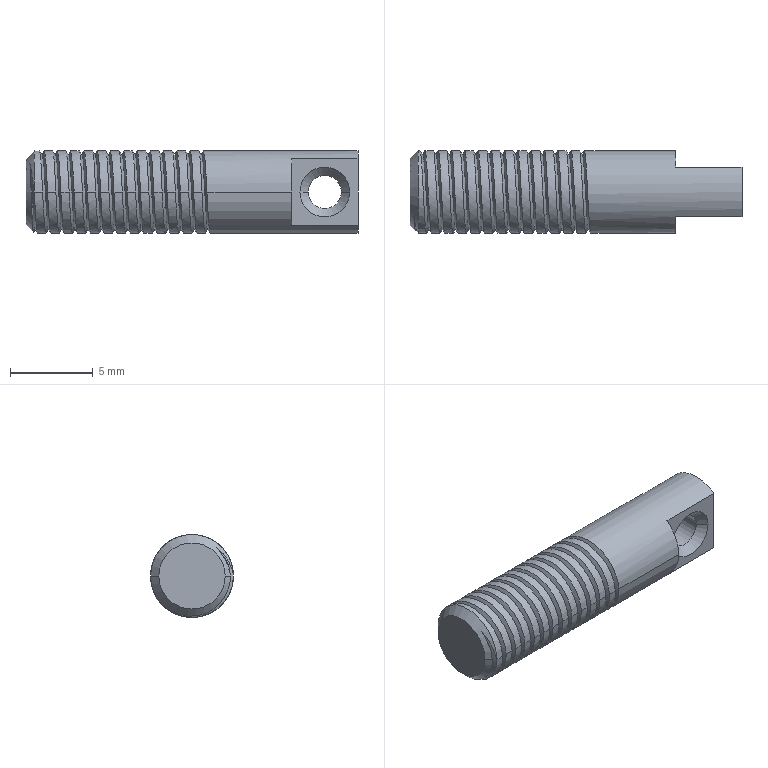Part | NX | 1 solid | 52 faces | box 20 x 5 x 5 mm | volume 349.207 mm3 | cylinder 31 | spline 8 | plane 7 | cone 6 | commonest cylinder face diameters 5 x29 2 x2